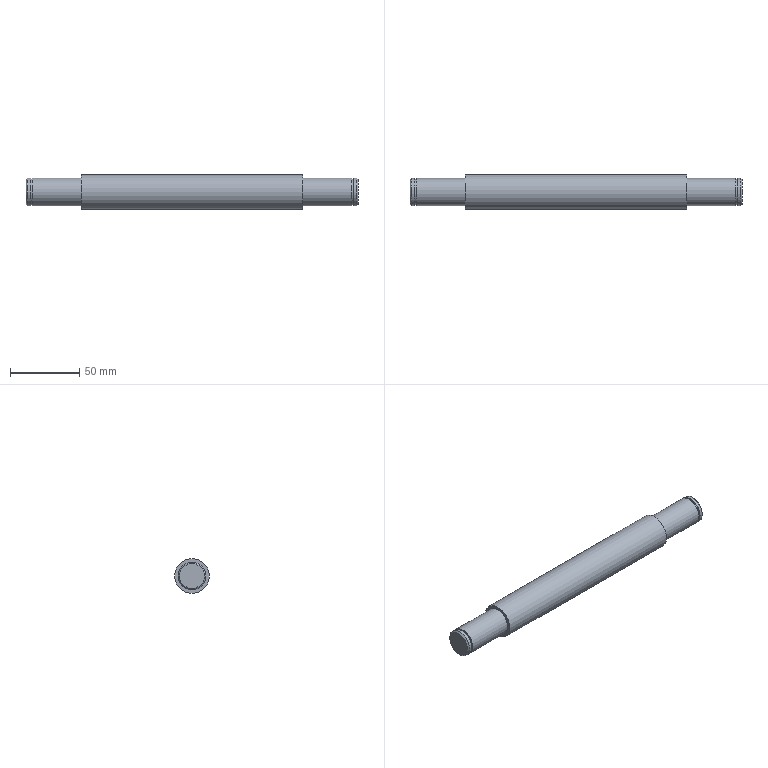Part | STEP file | Shaft2 | 1 solid | 17 faces | box 240 x 25 x 25 mm | volume 103493 mm3 | plane 8 | cylinder 7 | cone 2 | commonest cylinder face diameters 20 x4 18.35 x2 25 x1
STEP:
#1=CARTESIAN_POINT('',(0.,0.,0.));
#2=DIRECTION('',(0.,0.,1.));
#3=DIRECTION('',(1.,0.,0.));
#4=AXIS2_PLACEMENT_3D('',#1,#2,#3);
#5=CARTESIAN_POINT('',(239.,10.,0.));
#6=VERTEX_POINT('',#5);
#7=CARTESIAN_POINT('',(239.,0.,0.));
#8=DIRECTION('',(1.,0.,0.));
#9=DIRECTION('',(0.,-1.,0.));
#10=AXIS2_PLACEMENT_3D('',#7,#8,#9);
#11=CIRCLE('',#10,10.);
#12=CARTESIAN_POINT('',(239.5,0.,0.));
#13=DIRECTION('',(-1.,0.,0.));
#14=DIRECTION('',(0.,-1.,0.));
#15=AXIS2_PLACEMENT_3D('',#12,#13,#14);
#16=CONICAL_SURFACE('',#15,9.5,0.7854);
#17=CARTESIAN_POINT('',(12.566,0.5));
#18=DIRECTION('',(-1.,0.));
#19=VECTOR('',#18,1.);
#20=LINE('',#17,#19);
#21=(GEOMETRIC_REPRESENTATION_CONTEXT(2)PARAMETRIC_REPRESENTATION_CONTEXT()REPRESENTATION_CONTEXT('',''));
#22=DEFINITIONAL_REPRESENTATION('',(#20),#21);
#23=PCURVE('',#16,#22);
#24=CARTESIAN_POINT('',(220.,0.,0.));
#25=DIRECTION('',(1.,0.,0.));
#26=DIRECTION('',(0.,1.,0.));
#27=AXIS2_PLACEMENT_3D('',#24,#25,#26);
#28=CYLINDRICAL_SURFACE('',#27,10.);
#29=CARTESIAN_POINT('',(-3.142,19.));
#30=DIRECTION('',(1.,0.));
#31=VECTOR('',#30,1.);
#32=LINE('',#29,#31);
#33=(GEOMETRIC_REPRESENTATION_CONTEXT(2)PARAMETRIC_REPRESENTATION_CONTEXT()REPRESENTATION_CONTEXT('',''));
#34=DEFINITIONAL_REPRESENTATION('',(#32),#33);
#35=PCURVE('',#28,#34);
#36=SURFACE_CURVE('',#11,(#23,#35),.PCURVE_S1.);
#37=EDGE_CURVE('',#6,#6,#36,.T.);
#38=ORIENTED_EDGE('',*,*,#37,.T.);
#39=CARTESIAN_POINT('',(240.,9.,0.));
#40=VERTEX_POINT('',#39);
#41=CARTESIAN_POINT('',(240.,9.,0.));
#42=CARTESIAN_POINT('',(239.,10.,0.));
#43=B_SPLINE_CURVE_WITH_KNOTS('',1,(#41,#42),.UNSPECIFIED.,.F.,.F.,(2,2),(-0.7071,0.7071),.PIECEWISE_BEZIER_KNOTS.);
#44=CARTESIAN_POINT('',(3.142,0.));
#45=DIRECTION('',(0.,1.));
#46=VECTOR('',#45,1.);
#47=LINE('',#44,#46);
#48=(GEOMETRIC_REPRESENTATION_CONTEXT(2)PARAMETRIC_REPRESENTATION_CONTEXT()REPRESENTATION_CONTEXT('',''));
#49=DEFINITIONAL_REPRESENTATION('',(#47),#48);
#50=PCURVE('',#16,#49);
#51=CARTESIAN_POINT('',(9.425,0.));
#52=DIRECTION('',(0.,1.));
#53=VECTOR('',#52,1.);
#54=LINE('',#51,#53);
#55=(GEOMETRIC_REPRESENTATION_CONTEXT(2)PARAMETRIC_REPRESENTATION_CONTEXT()REPRESENTATION_CONTEXT('',''));
#56=DEFINITIONAL_REPRESENTATION('',(#54),#55);
#57=PCURVE('',#16,#56);
#58=SEAM_CURVE('',#43,(#50,#57),.PCURVE_S1.);
#59=EDGE_CURVE('',#40,#6,#58,.T.);
#60=ORIENTED_EDGE('',*,*,#59,.F.);
#61=CARTESIAN_POINT('',(240.,0.,0.));
#62=DIRECTION('',(-1.,0.,0.));
#63=DIRECTION('',(0.,-1.,0.));
#64=AXIS2_PLACEMENT_3D('',#61,#62,#63);
#65=CIRCLE('',#64,9.);
#66=CARTESIAN_POINT('',(0.,-0.5));
#67=DIRECTION('',(1.,0.));
#68=VECTOR('',#67,1.);
#69=LINE('',#66,#68);
#70=(GEOMETRIC_REPRESENTATION_CONTEXT(2)PARAMETRIC_REPRESENTATION_CONTEXT()REPRESENTATION_CONTEXT('',''));
#71=DEFINITIONAL_REPRESENTATION('',(#69),#70);
#72=PCURVE('',#16,#71);
#73=CARTESIAN_POINT('',(240.,0.,0.));
#74=DIRECTION('',(1.,0.,0.));
#75=DIRECTION('',(0.,0.,-1.));
#76=AXIS2_PLACEMENT_3D('',#73,#74,#75);
#77=PLANE('',#76);
#78=CARTESIAN_POINT('',(0.,-9.));
#79=CARTESIAN_POINT('',(-15.588,-9.));
#80=CARTESIAN_POINT('',(-7.794,4.5));
#81=CARTESIAN_POINT('',(0.,18.));
#82=CARTESIAN_POINT('',(7.794,4.5));
#83=CARTESIAN_POINT('',(15.588,-9.));
#84=CARTESIAN_POINT('',(0.,-9.));
#85=(BOUNDED_CURVE()B_SPLINE_CURVE(2,(#78,#79,#80,#81,#82,#83,#84),.UNSPECIFIED.,.T.,.F.)B_SPLINE_CURVE_WITH_KNOTS((1,2,2,2,2,1),(-2.094,0.,2.094,4.189,6.283,8.378),.UNSPECIFIED.)CURVE()GEOMETRIC_REPRESENTATION_ITEM()RATIONAL_B_SPLINE_CURVE((1.,0.5,1.,0.5,1.,0.5,1.))REPRESENTATION_ITEM(''));
#86=(GEOMETRIC_REPRESENTATION_CONTEXT(2)PARAMETRIC_REPRESENTATION_CONTEXT()REPRESENTATION_CONTEXT('',''));
#87=DEFINITIONAL_REPRESENTATION('',(#85),#86);
#88=PCURVE('',#77,#87);
#89=SURFACE_CURVE('',#65,(#72,#88),.PCURVE_S1.);
#90=EDGE_CURVE('',#40,#40,#89,.T.);
#91=ORIENTED_EDGE('',*,*,#90,.T.);
#92=ORIENTED_EDGE('',*,*,#59,.T.);
#93=EDGE_LOOP('',(#38,#60,#91,#92));
#94=FACE_BOUND('',#93,.T.);
#95=ADVANCED_FACE('',(#94),#16,.T.);
#96=CARTESIAN_POINT('',(236.789,10.,0.));
#97=VERTEX_POINT('',#96);
#98=CARTESIAN_POINT('',(236.789,0.,0.));
#99=DIRECTION('',(1.,0.,0.));
#100=DIRECTION('',(0.,1.,0.));
#101=AXIS2_PLACEMENT_3D('',#98,#99,#100);
#102=CIRCLE('',#101,10.);
#103=CARTESIAN_POINT('',(0.,16.789));
#104=DIRECTION('',(1.,0.));
#105=VECTOR('',#104,1.);
#106=LINE('',#103,#105);
#107=(GEOMETRIC_REPRESENTATION_CONTEXT(2)PARAMETRIC_REPRESENTATION_CONTEXT()REPRESENTATION_CONTEXT('',''));
#108=DEFINITIONAL_REPRESENTATION('',(#106),#107);
#109=PCURVE('',#28,#108);
#110=CARTESIAN_POINT('',(236.789,0.,0.));
#111=DIRECTION('',(-1.,0.,0.));
#112=DIRECTION('',(0.,0.,1.));
#113=AXIS2_PLACEMENT_3D('',#110,#111,#112);
#114=PLANE('',#113);
#115=CARTESIAN_POINT('',(0.,10.));
#116=CARTESIAN_POINT('',(17.321,10.));
#117=CARTESIAN_POINT('',(8.66,-5.));
#118=CARTESIAN_POINT('',(0.,-20.));
#119=CARTESIAN_POINT('',(-8.66,-5.));
#120=CARTESIAN_POINT('',(-17.321,10.));
#121=CARTESIAN_POINT('',(0.,10.));
#122=(BOUNDED_CURVE()B_SPLINE_CURVE(2,(#115,#116,#117,#118,#119,#120,#121),.UNSPECIFIED.,.T.,.F.)B_SPLINE_CURVE_WITH_KNOTS((1,2,2,2,2,1),(-2.094,0.,2.094,4.189,6.283,8.378),.UNSPECIFIED.)CURVE()GEOMETRIC_REPRESENTATION_ITEM()RATIONAL_B_SPLINE_CURVE((1.,0.5,1.,0.5,1.,0.5,1.))REPRESENTATION_ITEM(''));
#123=(GEOMETRIC_REPRESENTATION_CONTEXT(2)PARAMETRIC_REPRESENTATION_CONTEXT()REPRESENTATION_CONTEXT('',''));
#124=DEFINITIONAL_REPRESENTATION('',(#122),#123);
#125=PCURVE('',#114,#124);
#126=SURFACE_CURVE('',#102,(#109,#125),.PCURVE_S1.);
#127=EDGE_CURVE('',#97,#97,#126,.T.);
#128=ORIENTED_EDGE('',*,*,#127,.T.);
#129=CARTESIAN_POINT('',(236.789,10.,0.));
#130=CARTESIAN_POINT('',(239.,10.,0.));
#131=B_SPLINE_CURVE_WITH_KNOTS('',1,(#129,#130),.UNSPECIFIED.,.F.,.F.,(2,2),(16.789,19.),.PIECEWISE_BEZIER_KNOTS.);
#132=CARTESIAN_POINT('',(6.283,0.));
#133=DIRECTION('',(0.,1.));
#134=VECTOR('',#133,1.);
#135=LINE('',#132,#134);
#136=(GEOMETRIC_REPRESENTATION_CONTEXT(2)PARAMETRIC_REPRESENTATION_CONTEXT()REPRESENTATION_CONTEXT('',''));
#137=DEFINITIONAL_REPRESENTATION('',(#135),#136);
#138=PCURVE('',#28,#137);
#139=CARTESIAN_POINT('',(0.,0.));
#140=DIRECTION('',(0.,1.));
#141=VECTOR('',#140,1.);
#142=LINE('',#139,#141);
#143=(GEOMETRIC_REPRESENTATION_CONTEXT(2)PARAMETRIC_REPRESENTATION_CONTEXT()REPRESENTATION_CONTEXT('',''));
#144=DEFINITIONAL_REPRESENTATION('',(#142),#143);
#145=PCURVE('',#28,#144);
#146=SEAM_CURVE('',#131,(#138,#145),.PCURVE_S1.);
#147=EDGE_CURVE('',#97,#6,#146,.T.);
#148=ORIENTED_EDGE('',*,*,#147,.T.);
#149=ORIENTED_EDGE('',*,*,#37,.F.);
#150=ORIENTED_EDGE('',*,*,#147,.F.);
#151=EDGE_LOOP('',(#128,#148,#149,#150));
#152=FACE_BOUND('',#151,.T.);
#153=ADVANCED_FACE('',(#152),#28,.T.);
#154=ORIENTED_EDGE('',*,*,#90,.F.);
#155=EDGE_LOOP('',(#154));
#156=FACE_BOUND('',#155,.T.);
#157=ADVANCED_FACE('',(#156),#77,.T.);
#158=CARTESIAN_POINT('',(0.,9.,0.));
#159=VERTEX_POINT('',#158);
#160=CARTESIAN_POINT('',(0.,0.,0.));
#161=DIRECTION('',(1.,0.,0.));
#162=DIRECTION('',(0.,-1.,0.));
#163=AXIS2_PLACEMENT_3D('',#160,#161,#162);
#164=CIRCLE('',#163,9.);
#165=CARTESIAN_POINT('',(0.5,0.,0.));
#166=DIRECTION('',(1.,0.,0.));
#167=DIRECTION('',(0.,-1.,0.));
#168=AXIS2_PLACEMENT_3D('',#165,#166,#167);
#169=CONICAL_SURFACE('',#168,9.5,0.7854);
#170=CARTESIAN_POINT('',(0.,-0.5));
#171=DIRECTION('',(1.,0.));
#172=VECTOR('',#171,1.);
#173=LINE('',#170,#172);
#174=(GEOMETRIC_REPRESENTATION_CONTEXT(2)PARAMETRIC_REPRESENTATION_CONTEXT()REPRESENTATION_CONTEXT('',''));
#175=DEFINITIONAL_REPRESENTATION('',(#173),#174);
#176=PCURVE('',#169,#175);
#177=CARTESIAN_POINT('',(0.,10.,0.));
#178=DIRECTION('',(-1.,0.,0.));
#179=DIRECTION('',(0.,0.,1.));
#180=AXIS2_PLACEMENT_3D('',#177,#178,#179);
#181=PLANE('',#180);
#182=CARTESIAN_POINT('',(0.,-19.));
#183=CARTESIAN_POINT('',(-15.588,-19.));
#184=CARTESIAN_POINT('',(-7.794,-5.5));
#185=CARTESIAN_POINT('',(0.,8.));
#186=CARTESIAN_POINT('',(7.794,-5.5));
#187=CARTESIAN_POINT('',(15.588,-19.));
#188=CARTESIAN_POINT('',(0.,-19.));
#189=(BOUNDED_CURVE()B_SPLINE_CURVE(2,(#182,#183,#184,#185,#186,#187,#188),.UNSPECIFIED.,.T.,.F.)B_SPLINE_CURVE_WITH_KNOTS((1,2,2,2,2,1),(-2.094,0.,2.094,4.189,6.283,8.378),.UNSPECIFIED.)CURVE()GEOMETRIC_REPRESENTATION_ITEM()RATIONAL_B_SPLINE_CURVE((1.,0.5,1.,0.5,1.,0.5,1.))REPRESENTATION_ITEM(''));
#190=(GEOMETRIC_REPRESENTATION_CONTEXT(2)PARAMETRIC_REPRESENTATION_CONTEXT()REPRESENTATION_CONTEXT('',''));
#191=DEFINITIONAL_REPRESENTATION('',(#189),#190);
#192=PCURVE('',#181,#191);
#193=SURFACE_CURVE('',#164,(#176,#192),.PCURVE_S1.);
#194=EDGE_CURVE('',#159,#159,#193,.T.);
#195=ORIENTED_EDGE('',*,*,#194,.T.);
#196=CARTESIAN_POINT('',(1.,10.,0.));
#197=VERTEX_POINT('',#196);
#198=CARTESIAN_POINT('',(0.,9.,0.));
#199=CARTESIAN_POINT('',(1.,10.,0.));
#200=B_SPLINE_CURVE_WITH_KNOTS('',1,(#198,#199),.UNSPECIFIED.,.F.,.F.,(2,2),(-0.7071,0.7071),.PIECEWISE_BEZIER_KNOTS.);
#201=CARTESIAN_POINT('',(9.425,0.));
#202=DIRECTION('',(0.,1.));
#203=VECTOR('',#202,1.);
#204=LINE('',#201,#203);
#205=(GEOMETRIC_REPRESENTATION_CONTEXT(2)PARAMETRIC_REPRESENTATION_CONTEXT()REPRESENTATION_CONTEXT('',''));
#206=DEFINITIONAL_REPRESENTATION('',(#204),#205);
#207=PCURVE('',#169,#206);
#208=CARTESIAN_POINT('',(3.142,0.));
#209=DIRECTION('',(0.,1.));
#210=VECTOR('',#209,1.);
#211=LINE('',#208,#210);
#212=(GEOMETRIC_REPRESENTATION_CONTEXT(2)PARAMETRIC_REPRESENTATION_CONTEXT()REPRESENTATION_CONTEXT('',''));
#213=DEFINITIONAL_REPRESENTATION('',(#211),#212);
#214=PCURVE('',#169,#213);
#215=SEAM_CURVE('',#200,(#207,#214),.PCURVE_S1.);
#216=EDGE_CURVE('',#159,#197,#215,.T.);
#217=ORIENTED_EDGE('',*,*,#216,.T.);
#218=CARTESIAN_POINT('',(1.,0.,0.));
#219=DIRECTION('',(-1.,0.,0.));
#220=DIRECTION('',(0.,-1.,0.));
#221=AXIS2_PLACEMENT_3D('',#218,#219,#220);
#222=CIRCLE('',#221,10.);
#223=CARTESIAN_POINT('',(12.566,0.5));
#224=DIRECTION('',(-1.,0.));
#225=VECTOR('',#224,1.);
#226=LINE('',#223,#225);
#227=(GEOMETRIC_REPRESENTATION_CONTEXT(2)PARAMETRIC_REPRESENTATION_CONTEXT()REPRESENTATION_CONTEXT('',''));
#228=DEFINITIONAL_REPRESENTATION('',(#226),#227);
#229=PCURVE('',#169,#228);
#230=CARTESIAN_POINT('',(20.,0.,0.));
#231=DIRECTION('',(1.,0.,0.));
#232=DIRECTION('',(0.,1.,0.));
#233=AXIS2_PLACEMENT_3D('',#230,#231,#232);
#234=CYLINDRICAL_SURFACE('',#233,10.);
#235=CARTESIAN_POINT('',(9.425,-19.));
#236=DIRECTION('',(-1.,0.));
#237=VECTOR('',#236,1.);
#238=LINE('',#235,#237);
#239=(GEOMETRIC_REPRESENTATION_CONTEXT(2)PARAMETRIC_REPRESENTATION_CONTEXT()REPRESENTATION_CONTEXT('',''));
#240=DEFINITIONAL_REPRESENTATION('',(#238),#239);
#241=PCURVE('',#234,#240);
#242=SURFACE_CURVE('',#222,(#229,#241),.PCURVE_S1.);
#243=EDGE_CURVE('',#197,#197,#242,.T.);
#244=ORIENTED_EDGE('',*,*,#243,.T.);
#245=ORIENTED_EDGE('',*,*,#216,.F.);
#246=EDGE_LOOP('',(#195,#217,#244,#245));
#247=FACE_BOUND('',#246,.T.);
#248=ADVANCED_FACE('',(#247),#169,.T.);
#249=CARTESIAN_POINT('',(3.291,10.,0.));
#250=VERTEX_POINT('',#249);
#251=CARTESIAN_POINT('',(3.291,0.,0.));
#252=DIRECTION('',(-1.,0.,0.));
#253=DIRECTION('',(0.,1.,0.));
#254=AXIS2_PLACEMENT_3D('',#251,#252,#253);
#255=CIRCLE('',#254,10.);
#256=CARTESIAN_POINT('',(6.283,-16.709));
#257=DIRECTION('',(-1.,0.));
#258=VECTOR('',#257,1.);
#259=LINE('',#256,#258);
#260=(GEOMETRIC_REPRESENTATION_CONTEXT(2)PARAMETRIC_REPRESENTATION_CONTEXT()REPRESENTATION_CONTEXT('',''));
#261=DEFINITIONAL_REPRESENTATION('',(#259),#260);
#262=PCURVE('',#234,#261);
#263=CARTESIAN_POINT('',(3.291,0.,0.));
#264=DIRECTION('',(-1.,0.,0.));
#265=DIRECTION('',(0.,0.,1.));
#266=AXIS2_PLACEMENT_3D('',#263,#264,#265);
#267=PLANE('',#266);
#268=CARTESIAN_POINT('',(0.,0.));
#269=DIRECTION('',(0.,1.));
#270=AXIS2_PLACEMENT_2D('',#268,#269);
#271=CIRCLE('',#270,10.);
#272=(GEOMETRIC_REPRESENTATION_CONTEXT(2)PARAMETRIC_REPRESENTATION_CONTEXT()REPRESENTATION_CONTEXT('',''));
#273=DEFINITIONAL_REPRESENTATION('',(#271),#272);
#274=PCURVE('',#267,#273);
#275=SURFACE_CURVE('',#255,(#262,#274),.PCURVE_S1.);
#276=EDGE_CURVE('',#250,#250,#275,.T.);
#277=ORIENTED_EDGE('',*,*,#276,.T.);
#278=CARTESIAN_POINT('',(1.,10.,0.));
#279=CARTESIAN_POINT('',(3.291,10.,0.));
#280=B_SPLINE_CURVE_WITH_KNOTS('',1,(#278,#279),.UNSPECIFIED.,.F.,.F.,(2,2),(-19.,-16.709),.PIECEWISE_BEZIER_KNOTS.);
#281=CARTESIAN_POINT('',(0.,0.));
#282=DIRECTION('',(0.,1.));
#283=VECTOR('',#282,1.);
#284=LINE('',#281,#283);
#285=(GEOMETRIC_REPRESENTATION_CONTEXT(2)PARAMETRIC_REPRESENTATION_CONTEXT()REPRESENTATION_CONTEXT('',''));
#286=DEFINITIONAL_REPRESENTATION('',(#284),#285);
#287=PCURVE('',#234,#286);
#288=CARTESIAN_POINT('',(6.283,0.));
#289=DIRECTION('',(0.,1.));
#290=VECTOR('',#289,1.);
#291=LINE('',#288,#290);
#292=(GEOMETRIC_REPRESENTATION_CONTEXT(2)PARAMETRIC_REPRESENTATION_CONTEXT()REPRESENTATION_CONTEXT('',''));
#293=DEFINITIONAL_REPRESENTATION('',(#291),#292);
#294=PCURVE('',#234,#293);
#295=SEAM_CURVE('',#280,(#287,#294),.PCURVE_S1.);
#296=EDGE_CURVE('',#197,#250,#295,.T.);
#297=ORIENTED_EDGE('',*,*,#296,.F.);
#298=ORIENTED_EDGE('',*,*,#243,.F.);
#299=ORIENTED_EDGE('',*,*,#296,.T.);
#300=EDGE_LOOP('',(#277,#297,#298,#299));
#301=FACE_BOUND('',#300,.T.);
#302=ADVANCED_FACE('',(#301),#234,.T.);
#303=ORIENTED_EDGE('',*,*,#194,.F.);
#304=EDGE_LOOP('',(#303));
#305=FACE_BOUND('',#304,.T.);
#306=ADVANCED_FACE('',(#305),#181,.T.);
#307=CARTESIAN_POINT('',(4.491,9.175,0.));
#308=VERTEX_POINT('',#307);
#309=CARTESIAN_POINT('',(4.491,0.,0.));
#310=DIRECTION('',(-1.,0.,0.));
#311=DIRECTION('',(0.,-1.,0.));
#312=AXIS2_PLACEMENT_3D('',#309,#310,#311);
#313=CIRCLE('',#312,9.175);
#314=CARTESIAN_POINT('',(3.891,0.,0.));
#315=DIRECTION('',(-1.,0.,0.));
#316=DIRECTION('',(0.,-1.,0.));
#317=AXIS2_PLACEMENT_3D('',#314,#315,#316);
#318=CYLINDRICAL_SURFACE('',#317,9.175);
#319=CARTESIAN_POINT('',(0.,-0.6));
#320=DIRECTION('',(1.,0.));
#321=VECTOR('',#320,1.);
#322=LINE('',#319,#321);
#323=(GEOMETRIC_REPRESENTATION_CONTEXT(2)PARAMETRIC_REPRESENTATION_CONTEXT()REPRESENTATION_CONTEXT('',''));
#324=DEFINITIONAL_REPRESENTATION('',(#322),#323);
#325=PCURVE('',#318,#324);
#326=CARTESIAN_POINT('',(4.491,0.,0.));
#327=DIRECTION('',(-1.,0.,0.));
#328=DIRECTION('',(0.,0.,1.));
#329=AXIS2_PLACEMENT_3D('',#326,#327,#328);
#330=PLANE('',#329);
#331=CARTESIAN_POINT('',(0.,0.));
#332=DIRECTION('',(0.,-1.));
#333=AXIS2_PLACEMENT_2D('',#331,#332);
#334=CIRCLE('',#333,9.175);
#335=(GEOMETRIC_REPRESENTATION_CONTEXT(2)PARAMETRIC_REPRESENTATION_CONTEXT()REPRESENTATION_CONTEXT('',''));
#336=DEFINITIONAL_REPRESENTATION('',(#334),#335);
#337=PCURVE('',#330,#336);
#338=SURFACE_CURVE('',#313,(#325,#337),.PCURVE_S1.);
#339=EDGE_CURVE('',#308,#308,#338,.T.);
#340=ORIENTED_EDGE('',*,*,#339,.T.);
#341=CARTESIAN_POINT('',(3.291,9.175,0.));
#342=VERTEX_POINT('',#341);
#343=CARTESIAN_POINT('',(4.491,9.175,0.));
#344=CARTESIAN_POINT('',(3.291,9.175,0.));
#345=B_SPLINE_CURVE_WITH_KNOTS('',1,(#343,#344),.UNSPECIFIED.,.F.,.F.,(2,2),(-0.6,0.6),.PIECEWISE_BEZIER_KNOTS.);
#346=CARTESIAN_POINT('',(9.425,0.));
#347=DIRECTION('',(0.,1.));
#348=VECTOR('',#347,1.);
#349=LINE('',#346,#348);
#350=(GEOMETRIC_REPRESENTATION_CONTEXT(2)PARAMETRIC_REPRESENTATION_CONTEXT()REPRESENTATION_CONTEXT('',''));
#351=DEFINITIONAL_REPRESENTATION('',(#349),#350);
#352=PCURVE('',#318,#351);
#353=CARTESIAN_POINT('',(3.142,0.));
#354=DIRECTION('',(0.,1.));
#355=VECTOR('',#354,1.);
#356=LINE('',#353,#355);
#357=(GEOMETRIC_REPRESENTATION_CONTEXT(2)PARAMETRIC_REPRESENTATION_CONTEXT()REPRESENTATION_CONTEXT('',''));
#358=DEFINITIONAL_REPRESENTATION('',(#356),#357);
#359=PCURVE('',#318,#358);
#360=SEAM_CURVE('',#345,(#352,#359),.PCURVE_S1.);
#361=EDGE_CURVE('',#308,#342,#360,.T.);
#362=ORIENTED_EDGE('',*,*,#361,.T.);
#363=CARTESIAN_POINT('',(3.291,0.,0.));
#364=DIRECTION('',(1.,0.,0.));
#365=DIRECTION('',(0.,-1.,0.));
#366=AXIS2_PLACEMENT_3D('',#363,#364,#365);
#367=CIRCLE('',#366,9.175);
#368=CARTESIAN_POINT('',(12.566,0.6));
#369=DIRECTION('',(-1.,0.));
#370=VECTOR('',#369,1.);
#371=LINE('',#368,#370);
#372=(GEOMETRIC_REPRESENTATION_CONTEXT(2)PARAMETRIC_REPRESENTATION_CONTEXT()REPRESENTATION_CONTEXT('',''));
#373=DEFINITIONAL_REPRESENTATION('',(#371),#372);
#374=PCURVE('',#318,#373);
#375=CARTESIAN_POINT('',(0.,-9.175));
#376=CARTESIAN_POINT('',(-15.892,-9.175));
#377=CARTESIAN_POINT('',(-7.946,4.588));
#378=CARTESIAN_POINT('',(0.,18.35));
#379=CARTESIAN_POINT('',(7.946,4.588));
#380=CARTESIAN_POINT('',(15.892,-9.175));
#381=CARTESIAN_POINT('',(0.,-9.175));
#382=(BOUNDED_CURVE()B_SPLINE_CURVE(2,(#375,#376,#377,#378,#379,#380,#381),.UNSPECIFIED.,.T.,.F.)B_SPLINE_CURVE_WITH_KNOTS((1,2,2,2,2,1),(-2.094,0.,2.094,4.189,6.283,8.378),.UNSPECIFIED.)CURVE()GEOMETRIC_REPRESENTATION_ITEM()RATIONAL_B_SPLINE_CURVE((1.,0.5,1.,0.5,1.,0.5,1.))REPRESENTATION_ITEM(''));
#383=(GEOMETRIC_REPRESENTATION_CONTEXT(2)PARAMETRIC_REPRESENTATION_CONTEXT()REPRESENTATION_CONTEXT('',''));
#384=DEFINITIONAL_REPRESENTATION('',(#382),#383);
#385=PCURVE('',#267,#384);
#386=SURFACE_CURVE('',#367,(#374,#385),.PCURVE_S1.);
#387=EDGE_CURVE('',#342,#342,#386,.T.);
#388=ORIENTED_EDGE('',*,*,#387,.T.);
#389=ORIENTED_EDGE('',*,*,#361,.F.);
#390=EDGE_LOOP('',(#340,#362,#388,#389));
#391=FACE_BOUND('',#390,.T.);
#392=ADVANCED_FACE('',(#391),#318,.T.);
#393=CARTESIAN_POINT('',(4.491,10.,0.));
#394=VERTEX_POINT('',#393);
#395=CARTESIAN_POINT('',(4.491,0.,0.));
#396=DIRECTION('',(1.,0.,0.));
#397=DIRECTION('',(0.,1.,0.));
#398=AXIS2_PLACEMENT_3D('',#395,#396,#397);
#399=CIRCLE('',#398,10.);
#400=CARTESIAN_POINT('',(0.,10.));
#401=CARTESIAN_POINT('',(17.321,10.));
#402=CARTESIAN_POINT('',(8.66,-5.));
#403=CARTESIAN_POINT('',(0.,-20.));
#404=CARTESIAN_POINT('',(-8.66,-5.));
#405=CARTESIAN_POINT('',(-17.321,10.));
#406=CARTESIAN_POINT('',(0.,10.));
#407=(BOUNDED_CURVE()B_SPLINE_CURVE(2,(#400,#401,#402,#403,#404,#405,#406),.UNSPECIFIED.,.T.,.F.)B_SPLINE_CURVE_WITH_KNOTS((1,2,2,2,2,1),(-2.094,0.,2.094,4.189,6.283,8.378),.UNSPECIFIED.)CURVE()GEOMETRIC_REPRESENTATION_ITEM()RATIONAL_B_SPLINE_CURVE((1.,0.5,1.,0.5,1.,0.5,1.))REPRESENTATION_ITEM(''));
#408=(GEOMETRIC_REPRESENTATION_CONTEXT(2)PARAMETRIC_REPRESENTATION_CONTEXT()REPRESENTATION_CONTEXT('',''));
#409=DEFINITIONAL_REPRESENTATION('',(#407),#408);
#410=PCURVE('',#330,#409);
#411=CARTESIAN_POINT('',(20.,0.,0.));
#412=DIRECTION('',(1.,0.,0.));
#413=DIRECTION('',(0.,1.,0.));
#414=AXIS2_PLACEMENT_3D('',#411,#412,#413);
#415=CYLINDRICAL_SURFACE('',#414,10.);
#416=CARTESIAN_POINT('',(0.,-15.509));
#417=DIRECTION('',(1.,0.));
#418=VECTOR('',#417,1.);
#419=LINE('',#416,#418);
#420=(GEOMETRIC_REPRESENTATION_CONTEXT(2)PARAMETRIC_REPRESENTATION_CONTEXT()REPRESENTATION_CONTEXT('',''));
#421=DEFINITIONAL_REPRESENTATION('',(#419),#420);
#422=PCURVE('',#415,#421);
#423=SURFACE_CURVE('',#399,(#410,#422),.PCURVE_S1.);
#424=EDGE_CURVE('',#394,#394,#423,.T.);
#425=ORIENTED_EDGE('',*,*,#424,.F.);
#426=EDGE_LOOP('',(#425));
#427=FACE_BOUND('',#426,.T.);
#428=ORIENTED_EDGE('',*,*,#339,.F.);
#429=EDGE_LOOP('',(#428));
#430=FACE_BOUND('',#429,.T.);
#431=ADVANCED_FACE('',(#427,#430),#330,.T.);
#432=ORIENTED_EDGE('',*,*,#276,.F.);
#433=EDGE_LOOP('',(#432));
#434=FACE_BOUND('',#433,.T.);
#435=ORIENTED_EDGE('',*,*,#387,.F.);
#436=EDGE_LOOP('',(#435));
#437=FACE_BOUND('',#436,.T.);
#438=ADVANCED_FACE('',(#434,#437),#267,.F.);
#439=CARTESIAN_POINT('',(236.789,9.175,0.));
#440=VERTEX_POINT('',#439);
#441=CARTESIAN_POINT('',(236.789,0.,0.));
#442=DIRECTION('',(-1.,0.,0.));
#443=DIRECTION('',(0.,-1.,0.));
#444=AXIS2_PLACEMENT_3D('',#441,#442,#443);
#445=CIRCLE('',#444,9.175);
#446=CARTESIAN_POINT('',(236.189,0.,0.));
#447=DIRECTION('',(-1.,0.,0.));
#448=DIRECTION('',(0.,-1.,0.));
#449=AXIS2_PLACEMENT_3D('',#446,#447,#448);
#450=CYLINDRICAL_SURFACE('',#449,9.175);
#451=CARTESIAN_POINT('',(0.,-0.6));
#452=DIRECTION('',(1.,0.));
#453=VECTOR('',#452,1.);
#454=LINE('',#451,#453);
#455=(GEOMETRIC_REPRESENTATION_CONTEXT(2)PARAMETRIC_REPRESENTATION_CONTEXT()REPRESENTATION_CONTEXT('',''));
#456=DEFINITIONAL_REPRESENTATION('',(#454),#455);
#457=PCURVE('',#450,#456);
#458=CARTESIAN_POINT('',(0.,0.));
#459=DIRECTION('',(0.,-1.));
#460=AXIS2_PLACEMENT_2D('',#458,#459);
#461=CIRCLE('',#460,9.175);
#462=(GEOMETRIC_REPRESENTATION_CONTEXT(2)PARAMETRIC_REPRESENTATION_CONTEXT()REPRESENTATION_CONTEXT('',''));
#463=DEFINITIONAL_REPRESENTATION('',(#461),#462);
#464=PCURVE('',#114,#463);
#465=SURFACE_CURVE('',#445,(#457,#464),.PCURVE_S1.);
#466=EDGE_CURVE('',#440,#440,#465,.T.);
#467=ORIENTED_EDGE('',*,*,#466,.T.);
#468=CARTESIAN_POINT('',(235.589,9.175,0.));
#469=VERTEX_POINT('',#468);
#470=CARTESIAN_POINT('',(236.789,9.175,0.));
#471=CARTESIAN_POINT('',(235.589,9.175,0.));
#472=B_SPLINE_CURVE_WITH_KNOTS('',1,(#470,#471),.UNSPECIFIED.,.F.,.F.,(2,2),(-0.6,0.6),.PIECEWISE_BEZIER_KNOTS.);
#473=CARTESIAN_POINT('',(9.425,0.));
#474=DIRECTION('',(0.,1.));
#475=VECTOR('',#474,1.);
#476=LINE('',#473,#475);
#477=(GEOMETRIC_REPRESENTATION_CONTEXT(2)PARAMETRIC_REPRESENTATION_CONTEXT()REPRESENTATION_CONTEXT('',''));
#478=DEFINITIONAL_REPRESENTATION('',(#476),#477);
#479=PCURVE('',#450,#478);
#480=CARTESIAN_POINT('',(3.142,0.));
#481=DIRECTION('',(0.,1.));
#482=VECTOR('',#481,1.);
#483=LINE('',#480,#482);
#484=(GEOMETRIC_REPRESENTATION_CONTEXT(2)PARAMETRIC_REPRESENTATION_CONTEXT()REPRESENTATION_CONTEXT('',''));
#485=DEFINITIONAL_REPRESENTATION('',(#483),#484);
#486=PCURVE('',#450,#485);
#487=SEAM_CURVE('',#472,(#479,#486),.PCURVE_S1.);
#488=EDGE_CURVE('',#440,#469,#487,.T.);
#489=ORIENTED_EDGE('',*,*,#488,.T.);
#490=CARTESIAN_POINT('',(235.589,0.,0.));
#491=DIRECTION('',(1.,0.,0.));
#492=DIRECTION('',(0.,-1.,0.));
#493=AXIS2_PLACEMENT_3D('',#490,#491,#492);
#494=CIRCLE('',#493,9.175);
#495=CARTESIAN_POINT('',(12.566,0.6));
#496=DIRECTION('',(-1.,0.));
#497=VECTOR('',#496,1.);
#498=LINE('',#495,#497);
#499=(GEOMETRIC_REPRESENTATION_CONTEXT(2)PARAMETRIC_REPRESENTATION_CONTEXT()REPRESENTATION_CONTEXT('',''));
#500=DEFINITIONAL_REPRESENTATION('',(#498),#499);
#501=PCURVE('',#450,#500);
#502=CARTESIAN_POINT('',(235.589,0.,0.));
#503=DIRECTION('',(-1.,0.,0.));
#504=DIRECTION('',(0.,0.,1.));
#505=AXIS2_PLACEMENT_3D('',#502,#503,#504);
#506=PLANE('',#505);
#507=CARTESIAN_POINT('',(0.,-9.175));
#508=CARTESIAN_POINT('',(-15.892,-9.175));
#509=CARTESIAN_POINT('',(-7.946,4.588));
#510=CARTESIAN_POINT('',(0.,18.35));
#511=CARTESIAN_POINT('',(7.946,4.588));
#512=CARTESIAN_POINT('',(15.892,-9.175));
#513=CARTESIAN_POINT('',(0.,-9.175));
#514=(BOUNDED_CURVE()B_SPLINE_CURVE(2,(#507,#508,#509,#510,#511,#512,#513),.UNSPECIFIED.,.T.,.F.)B_SPLINE_CURVE_WITH_KNOTS((1,2,2,2,2,1),(-2.094,0.,2.094,4.189,6.283,8.378),.UNSPECIFIED.)CURVE()GEOMETRIC_REPRESENTATION_ITEM()RATIONAL_B_SPLINE_CURVE((1.,0.5,1.,0.5,1.,0.5,1.))REPRESENTATION_ITEM(''));
#515=(GEOMETRIC_REPRESENTATION_CONTEXT(2)PARAMETRIC_REPRESENTATION_CONTEXT()REPRESENTATION_CONTEXT('',''));
#516=DEFINITIONAL_REPRESENTATION('',(#514),#515);
#517=PCURVE('',#506,#516);
#518=SURFACE_CURVE('',#494,(#501,#517),.PCURVE_S1.);
#519=EDGE_CURVE('',#469,#469,#518,.T.);
#520=ORIENTED_EDGE('',*,*,#519,.T.);
#521=ORIENTED_EDGE('',*,*,#488,.F.);
#522=EDGE_LOOP('',(#467,#489,#520,#521));
#523=FACE_BOUND('',#522,.T.);
#524=ADVANCED_FACE('',(#523),#450,.T.);
#525=ORIENTED_EDGE('',*,*,#127,.F.);
#526=EDGE_LOOP('',(#525));
#527=FACE_BOUND('',#526,.T.);
#528=ORIENTED_EDGE('',*,*,#466,.F.);
#529=EDGE_LOOP('',(#528));
#530=FACE_BOUND('',#529,.T.);
#531=ADVANCED_FACE('',(#527,#530),#114,.T.);
#532=CARTESIAN_POINT('',(235.589,10.,0.));
#533=VERTEX_POINT('',#532);
#534=CARTESIAN_POINT('',(235.589,0.,0.));
#535=DIRECTION('',(-1.,0.,0.));
#536=DIRECTION('',(0.,1.,0.));
#537=AXIS2_PLACEMENT_3D('',#534,#535,#536);
#538=CIRCLE('',#537,10.);
#539=CARTESIAN_POINT('',(0.,0.));
#540=DIRECTION('',(0.,1.));
#541=AXIS2_PLACEMENT_2D('',#539,#540);
#542=CIRCLE('',#541,10.);
#543=(GEOMETRIC_REPRESENTATION_CONTEXT(2)PARAMETRIC_REPRESENTATION_CONTEXT()REPRESENTATION_CONTEXT('',''));
#544=DEFINITIONAL_REPRESENTATION('',(#542),#543);
#545=PCURVE('',#506,#544);
#546=CARTESIAN_POINT('',(220.,0.,0.));
#547=DIRECTION('',(1.,0.,0.));
#548=DIRECTION('',(0.,1.,0.));
#549=AXIS2_PLACEMENT_3D('',#546,#547,#548);
#550=CYLINDRICAL_SURFACE('',#549,10.);
#551=CARTESIAN_POINT('',(6.283,15.589));
#552=DIRECTION('',(-1.,0.));
#553=VECTOR('',#552,1.);
#554=LINE('',#551,#553);
#555=(GEOMETRIC_REPRESENTATION_CONTEXT(2)PARAMETRIC_REPRESENTATION_CONTEXT()REPRESENTATION_CONTEXT('',''));
#556=DEFINITIONAL_REPRESENTATION('',(#554),#555);
#557=PCURVE('',#550,#556);
#558=SURFACE_CURVE('',#538,(#545,#557),.PCURVE_S1.);
#559=EDGE_CURVE('',#533,#533,#558,.T.);
#560=ORIENTED_EDGE('',*,*,#559,.F.);
#561=EDGE_LOOP('',(#560));
#562=FACE_BOUND('',#561,.T.);
#563=ORIENTED_EDGE('',*,*,#519,.F.);
#564=EDGE_LOOP('',(#563));
#565=FACE_BOUND('',#564,.T.);
#566=ADVANCED_FACE('',(#562,#565),#506,.F.);
#567=CARTESIAN_POINT('',(200.,10.,0.));
#568=VERTEX_POINT('',#567);
#569=CARTESIAN_POINT('',(200.,0.,0.));
#570=DIRECTION('',(1.,0.,0.));
#571=DIRECTION('',(0.,0.,-1.));
#572=AXIS2_PLACEMENT_3D('',#569,#570,#571);
#573=CIRCLE('',#572,10.);
#574=CARTESIAN_POINT('',(-1.571,-20.));
#575=DIRECTION('',(1.,0.));
#576=VECTOR('',#575,1.);
#577=LINE('',#574,#576);
#578=(GEOMETRIC_REPRESENTATION_CONTEXT(2)PARAMETRIC_REPRESENTATION_CONTEXT()REPRESENTATION_CONTEXT('',''));
#579=DEFINITIONAL_REPRESENTATION('',(#577),#578);
#580=PCURVE('',#550,#579);
#581=CARTESIAN_POINT('',(200.,10.,0.));
#582=DIRECTION('',(1.,0.,0.));
#583=DIRECTION('',(0.,0.,-1.));
#584=AXIS2_PLACEMENT_3D('',#581,#582,#583);
#585=PLANE('',#584);
#586=CARTESIAN_POINT('',(0.,-10.));
#587=DIRECTION('',(1.,0.));
#588=AXIS2_PLACEMENT_2D('',#586,#587);
#589=CIRCLE('',#588,10.);
#590=(GEOMETRIC_REPRESENTATION_CONTEXT(2)PARAMETRIC_REPRESENTATION_CONTEXT()REPRESENTATION_CONTEXT('',''));
#591=DEFINITIONAL_REPRESENTATION('',(#589),#590);
#592=PCURVE('',#585,#591);
#593=SURFACE_CURVE('',#573,(#580,#592),.PCURVE_S1.);
#594=EDGE_CURVE('',#568,#568,#593,.T.);
#595=ORIENTED_EDGE('',*,*,#594,.T.);
#596=CARTESIAN_POINT('',(200.,10.,0.));
#597=CARTESIAN_POINT('',(235.589,10.,0.));
#598=B_SPLINE_CURVE_WITH_KNOTS('',1,(#596,#597),.UNSPECIFIED.,.F.,.F.,(2,2),(-20.,15.589),.PIECEWISE_BEZIER_KNOTS.);
#599=CARTESIAN_POINT('',(6.283,0.));
#600=DIRECTION('',(0.,1.));
#601=VECTOR('',#600,1.);
#602=LINE('',#599,#601);
#603=(GEOMETRIC_REPRESENTATION_CONTEXT(2)PARAMETRIC_REPRESENTATION_CONTEXT()REPRESENTATION_CONTEXT('',''));
#604=DEFINITIONAL_REPRESENTATION('',(#602),#603);
#605=PCURVE('',#550,#604);
#606=CARTESIAN_POINT('',(0.,0.));
#607=DIRECTION('',(0.,1.));
#608=VECTOR('',#607,1.);
#609=LINE('',#606,#608);
#610=(GEOMETRIC_REPRESENTATION_CONTEXT(2)PARAMETRIC_REPRESENTATION_CONTEXT()REPRESENTATION_CONTEXT('',''));
#611=DEFINITIONAL_REPRESENTATION('',(#609),#610);
#612=PCURVE('',#550,#611);
#613=SEAM_CURVE('',#598,(#605,#612),.PCURVE_S1.);
#614=EDGE_CURVE('',#568,#533,#613,.T.);
#615=ORIENTED_EDGE('',*,*,#614,.T.);
#616=ORIENTED_EDGE('',*,*,#559,.T.);
#617=ORIENTED_EDGE('',*,*,#614,.F.);
#618=EDGE_LOOP('',(#595,#615,#616,#617));
#619=FACE_BOUND('',#618,.T.);
#620=ADVANCED_FACE('',(#619),#550,.T.);
#621=CARTESIAN_POINT('',(40.,12.5,0.));
#622=VERTEX_POINT('',#621);
#623=CARTESIAN_POINT('',(40.,0.,0.));
#624=DIRECTION('',(1.,0.,0.));
#625=DIRECTION('',(0.,0.,-1.));
#626=AXIS2_PLACEMENT_3D('',#623,#624,#625);
#627=CIRCLE('',#626,12.5);
#628=CARTESIAN_POINT('',(40.,12.5,0.));
#629=DIRECTION('',(-1.,0.,0.));
#630=DIRECTION('',(0.,0.,1.));
#631=AXIS2_PLACEMENT_3D('',#628,#629,#630);
#632=PLANE('',#631);
#633=CARTESIAN_POINT('',(-12.5,-12.5));
#634=CARTESIAN_POINT('',(-12.5,9.151));
#635=CARTESIAN_POINT('',(6.25,-1.675));
#636=CARTESIAN_POINT('',(25.,-12.5));
#637=CARTESIAN_POINT('',(6.25,-23.325));
#638=CARTESIAN_POINT('',(-12.5,-34.151));
#639=CARTESIAN_POINT('',(-12.5,-12.5));
#640=(BOUNDED_CURVE()B_SPLINE_CURVE(2,(#633,#634,#635,#636,#637,#638,#639),.UNSPECIFIED.,.T.,.F.)B_SPLINE_CURVE_WITH_KNOTS((1,2,2,2,2,1),(-2.094,0.,2.094,4.189,6.283,8.378),.UNSPECIFIED.)CURVE()GEOMETRIC_REPRESENTATION_ITEM()RATIONAL_B_SPLINE_CURVE((1.,0.5,1.,0.5,1.,0.5,1.))REPRESENTATION_ITEM(''));
#641=(GEOMETRIC_REPRESENTATION_CONTEXT(2)PARAMETRIC_REPRESENTATION_CONTEXT()REPRESENTATION_CONTEXT('',''));
#642=DEFINITIONAL_REPRESENTATION('',(#640),#641);
#643=PCURVE('',#632,#642);
#644=CARTESIAN_POINT('',(120.,0.,0.));
#645=DIRECTION('',(1.,0.,0.));
#646=DIRECTION('',(0.,1.,0.));
#647=AXIS2_PLACEMENT_3D('',#644,#645,#646);
#648=CYLINDRICAL_SURFACE('',#647,12.5);
#649=CARTESIAN_POINT('',(-1.571,-80.));
#650=DIRECTION('',(1.,0.));
#651=VECTOR('',#650,1.);
#652=LINE('',#649,#651);
#653=(GEOMETRIC_REPRESENTATION_CONTEXT(2)PARAMETRIC_REPRESENTATION_CONTEXT()REPRESENTATION_CONTEXT('',''));
#654=DEFINITIONAL_REPRESENTATION('',(#652),#653);
#655=PCURVE('',#648,#654);
#656=SURFACE_CURVE('',#627,(#643,#655),.PCURVE_S1.);
#657=EDGE_CURVE('',#622,#622,#656,.T.);
#658=ORIENTED_EDGE('',*,*,#657,.F.);
#659=EDGE_LOOP('',(#658));
#660=FACE_BOUND('',#659,.T.);
#661=CARTESIAN_POINT('',(40.,10.,0.));
#662=VERTEX_POINT('',#661);
#663=CARTESIAN_POINT('',(40.,0.,0.));
#664=DIRECTION('',(1.,0.,0.));
#665=DIRECTION('',(0.,0.,-1.));
#666=AXIS2_PLACEMENT_3D('',#663,#664,#665);
#667=CIRCLE('',#666,10.);
#668=CARTESIAN_POINT('',(-10.,-12.5));
#669=CARTESIAN_POINT('',(-10.,4.821));
#670=CARTESIAN_POINT('',(5.,-3.84));
#671=CARTESIAN_POINT('',(20.,-12.5));
#672=CARTESIAN_POINT('',(5.,-21.16));
#673=CARTESIAN_POINT('',(-10.,-29.821));
#674=CARTESIAN_POINT('',(-10.,-12.5));
#675=(BOUNDED_CURVE()B_SPLINE_CURVE(2,(#668,#669,#670,#671,#672,#673,#674),.UNSPECIFIED.,.T.,.F.)B_SPLINE_CURVE_WITH_KNOTS((1,2,2,2,2,1),(-2.094,0.,2.094,4.189,6.283,8.378),.UNSPECIFIED.)CURVE()GEOMETRIC_REPRESENTATION_ITEM()RATIONAL_B_SPLINE_CURVE((1.,0.5,1.,0.5,1.,0.5,1.))REPRESENTATION_ITEM(''));
#676=(GEOMETRIC_REPRESENTATION_CONTEXT(2)PARAMETRIC_REPRESENTATION_CONTEXT()REPRESENTATION_CONTEXT('',''));
#677=DEFINITIONAL_REPRESENTATION('',(#675),#676);
#678=PCURVE('',#632,#677);
#679=CARTESIAN_POINT('',(-1.571,20.));
#680=DIRECTION('',(1.,0.));
#681=VECTOR('',#680,1.);
#682=LINE('',#679,#681);
#683=(GEOMETRIC_REPRESENTATION_CONTEXT(2)PARAMETRIC_REPRESENTATION_CONTEXT()REPRESENTATION_CONTEXT('',''));
#684=DEFINITIONAL_REPRESENTATION('',(#682),#683);
#685=PCURVE('',#415,#684);
#686=SURFACE_CURVE('',#667,(#678,#685),.PCURVE_S1.);
#687=EDGE_CURVE('',#662,#662,#686,.T.);
#688=ORIENTED_EDGE('',*,*,#687,.T.);
#689=EDGE_LOOP('',(#688));
#690=FACE_BOUND('',#689,.T.);
#691=ADVANCED_FACE('',(#660,#690),#632,.T.);
#692=CARTESIAN_POINT('',(200.,12.5,0.));
#693=VERTEX_POINT('',#692);
#694=CARTESIAN_POINT('',(200.,0.,0.));
#695=DIRECTION('',(1.,0.,0.));
#696=DIRECTION('',(0.,0.,-1.));
#697=AXIS2_PLACEMENT_3D('',#694,#695,#696);
#698=CIRCLE('',#697,12.5);
#699=CARTESIAN_POINT('',(-1.571,80.));
#700=DIRECTION('',(1.,0.));
#701=VECTOR('',#700,1.);
#702=LINE('',#699,#701);
#703=(GEOMETRIC_REPRESENTATION_CONTEXT(2)PARAMETRIC_REPRESENTATION_CONTEXT()REPRESENTATION_CONTEXT('',''));
#704=DEFINITIONAL_REPRESENTATION('',(#702),#703);
#705=PCURVE('',#648,#704);
#706=CARTESIAN_POINT('',(0.,-10.));
#707=DIRECTION('',(1.,0.));
#708=AXIS2_PLACEMENT_2D('',#706,#707);
#709=CIRCLE('',#708,12.5);
#710=(GEOMETRIC_REPRESENTATION_CONTEXT(2)PARAMETRIC_REPRESENTATION_CONTEXT()REPRESENTATION_CONTEXT('',''));
#711=DEFINITIONAL_REPRESENTATION('',(#709),#710);
#712=PCURVE('',#585,#711);
#713=SURFACE_CURVE('',#698,(#705,#712),.PCURVE_S1.);
#714=EDGE_CURVE('',#693,#693,#713,.T.);
#715=ORIENTED_EDGE('',*,*,#714,.F.);
#716=CARTESIAN_POINT('',(40.,12.5,0.));
#717=CARTESIAN_POINT('',(200.,12.5,0.));
#718=B_SPLINE_CURVE_WITH_KNOTS('',1,(#716,#717),.UNSPECIFIED.,.F.,.F.,(2,2),(-80.,80.),.PIECEWISE_BEZIER_KNOTS.);
#719=CARTESIAN_POINT('',(0.,0.));
#720=DIRECTION('',(0.,1.));
#721=VECTOR('',#720,1.);
#722=LINE('',#719,#721);
#723=(GEOMETRIC_REPRESENTATION_CONTEXT(2)PARAMETRIC_REPRESENTATION_CONTEXT()REPRESENTATION_CONTEXT('',''));
#724=DEFINITIONAL_REPRESENTATION('',(#722),#723);
#725=PCURVE('',#648,#724);
#726=CARTESIAN_POINT('',(6.283,0.));
#727=DIRECTION('',(0.,1.));
#728=VECTOR('',#727,1.);
#729=LINE('',#726,#728);
#730=(GEOMETRIC_REPRESENTATION_CONTEXT(2)PARAMETRIC_REPRESENTATION_CONTEXT()REPRESENTATION_CONTEXT('',''));
#731=DEFINITIONAL_REPRESENTATION('',(#729),#730);
#732=PCURVE('',#648,#731);
#733=SEAM_CURVE('',#718,(#725,#732),.PCURVE_S1.);
#734=EDGE_CURVE('',#622,#693,#733,.T.);
#735=ORIENTED_EDGE('',*,*,#734,.F.);
#736=ORIENTED_EDGE('',*,*,#657,.T.);
#737=ORIENTED_EDGE('',*,*,#734,.T.);
#738=EDGE_LOOP('',(#715,#735,#736,#737));
#739=FACE_BOUND('',#738,.T.);
#740=ADVANCED_FACE('',(#739),#648,.T.);
#741=ORIENTED_EDGE('',*,*,#714,.T.);
#742=EDGE_LOOP('',(#741));
#743=FACE_BOUND('',#742,.T.);
#744=ORIENTED_EDGE('',*,*,#594,.F.);
#745=EDGE_LOOP('',(#744));
#746=FACE_BOUND('',#745,.T.);
#747=ADVANCED_FACE('',(#743,#746),#585,.T.);
#748=ORIENTED_EDGE('',*,*,#424,.T.);
#749=CARTESIAN_POINT('',(4.491,10.,0.));
#750=CARTESIAN_POINT('',(40.,10.,0.));
#751=B_SPLINE_CURVE_WITH_KNOTS('',1,(#749,#750),.UNSPECIFIED.,.F.,.F.,(2,2),(-15.509,20.),.PIECEWISE_BEZIER_KNOTS.);
#752=CARTESIAN_POINT('',(6.283,0.));
#753=DIRECTION('',(0.,1.));
#754=VECTOR('',#753,1.);
#755=LINE('',#752,#754);
#756=(GEOMETRIC_REPRESENTATION_CONTEXT(2)PARAMETRIC_REPRESENTATION_CONTEXT()REPRESENTATION_CONTEXT('',''));
#757=DEFINITIONAL_REPRESENTATION('',(#755),#756);
#758=PCURVE('',#415,#757);
#759=CARTESIAN_POINT('',(0.,0.));
#760=DIRECTION('',(0.,1.));
#761=VECTOR('',#760,1.);
#762=LINE('',#759,#761);
#763=(GEOMETRIC_REPRESENTATION_CONTEXT(2)PARAMETRIC_REPRESENTATION_CONTEXT()REPRESENTATION_CONTEXT('',''));
#764=DEFINITIONAL_REPRESENTATION('',(#762),#763);
#765=PCURVE('',#415,#764);
#766=SEAM_CURVE('',#751,(#758,#765),.PCURVE_S1.);
#767=EDGE_CURVE('',#394,#662,#766,.T.);
#768=ORIENTED_EDGE('',*,*,#767,.T.);
#769=ORIENTED_EDGE('',*,*,#687,.F.);
#770=ORIENTED_EDGE('',*,*,#767,.F.);
#771=EDGE_LOOP('',(#748,#768,#769,#770));
#772=FACE_BOUND('',#771,.T.);
#773=ADVANCED_FACE('',(#772),#415,.T.);
#774=CLOSED_SHELL('',(#95,#153,#157,#248,#302,#306,#392,#431,#438,#524,#531,#566,#620,#691,#740,#747,#773));
#775=MANIFOLD_SOLID_BREP('',#774);
#776=(LENGTH_UNIT()NAMED_UNIT(*)SI_UNIT(.MILLI.,.METRE.));
#777=UNCERTAINTY_MEASURE_WITH_UNIT(LENGTH_MEASURE(0.00001),#776,'','');
#778=(NAMED_UNIT(*)PLANE_ANGLE_UNIT()SI_UNIT($,.RADIAN.));
#779=(NAMED_UNIT(*)SI_UNIT($,.STERADIAN.)SOLID_ANGLE_UNIT());
#780=(GEOMETRIC_REPRESENTATION_CONTEXT(3)GLOBAL_UNCERTAINTY_ASSIGNED_CONTEXT((#777))GLOBAL_UNIT_ASSIGNED_CONTEXT((#776,#778,#779))REPRESENTATION_CONTEXT('',''));
#781=ADVANCED_BREP_SHAPE_REPRESENTATION('',(#4,#775),#780);